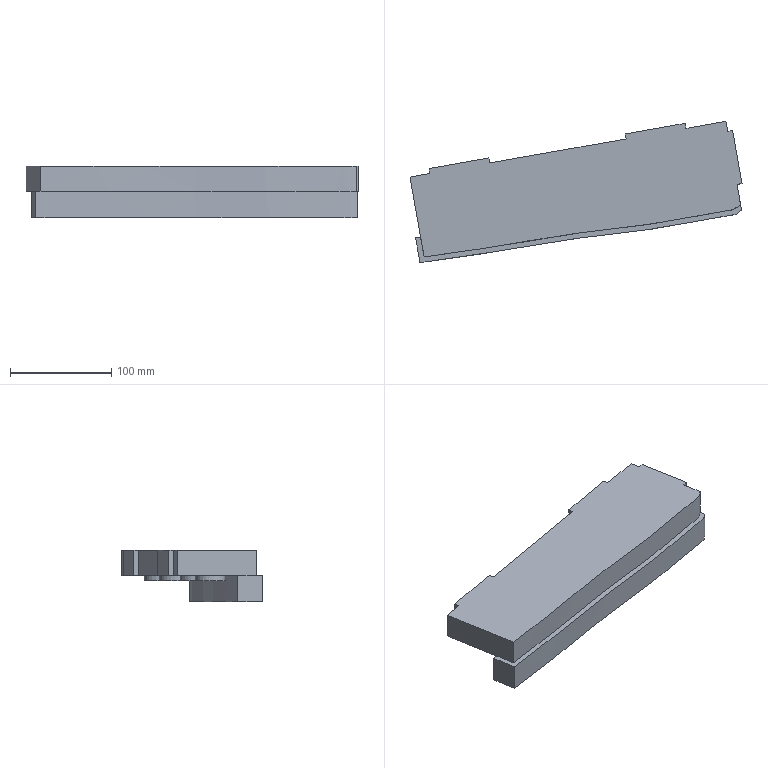Part | NX | features solid 2 | 1 solid | 33 faces | box 327.581 x 139.381 x 51 mm | volume 921541 mm3 | plane 25 | cylinder 5 | spline 3 | commonest cylinder face diameters 30 x5
STEP:
#1=CARTESIAN_POINT('',(309.963,629.515,45.));
#2=VERTEX_POINT('',#1);
#3=CARTESIAN_POINT('',(309.963,629.515,20.));
#4=VERTEX_POINT('',#3);
#5=CARTESIAN_POINT('',(309.963,629.515,51.));
#6=DIRECTION('',(0.,0.,-1.));
#7=VECTOR('',#6,1000.);
#8=LINE('',#5,#7);
#9=EDGE_CURVE('',#2,#4,#8,.T.);
#10=ORIENTED_EDGE('',*,*,#9,.F.);
#11=CARTESIAN_POINT('',(313.436,609.819,45.));
#12=VERTEX_POINT('',#11);
#13=CARTESIAN_POINT('',(310.85,624.485,45.));
#14=DIRECTION('',(-0.1736,0.9848,0.));
#15=VECTOR('',#14,1000.);
#16=LINE('',#13,#15);
#17=EDGE_CURVE('',#12,#2,#16,.T.);
#18=ORIENTED_EDGE('',*,*,#17,.F.);
#19=CARTESIAN_POINT('',(313.436,609.819,20.));
#20=VERTEX_POINT('',#19);
#21=CARTESIAN_POINT('',(313.436,609.819,32.5));
#22=DIRECTION('',(0.,0.,1.));
#23=VECTOR('',#22,1000.);
#24=LINE('',#21,#23);
#25=EDGE_CURVE('',#12,#20,#24,.F.);
#26=ORIENTED_EDGE('',*,*,#25,.T.);
#27=CARTESIAN_POINT('',(314.417,604.257,20.));
#28=VERTEX_POINT('',#27);
#29=CARTESIAN_POINT('',(314.417,604.257,20.));
#30=DIRECTION('',(0.1736,-0.9848,0.));
#31=VECTOR('',#30,1000.);
#32=LINE('',#29,#31);
#33=EDGE_CURVE('',#20,#28,#32,.T.);
#34=ORIENTED_EDGE('',*,*,#33,.T.);
#35=CARTESIAN_POINT('',(314.417,604.257,-6.));
#36=VERTEX_POINT('',#35);
#37=CARTESIAN_POINT('',(314.417,604.257,45.));
#38=DIRECTION('',(0.,0.,-1.));
#39=VECTOR('',#38,1000.);
#40=LINE('',#37,#39);
#41=EDGE_CURVE('',#28,#36,#40,.T.);
#42=ORIENTED_EDGE('',*,*,#41,.T.);
#43=CARTESIAN_POINT('',(310.85,624.485,-6.));
#44=VERTEX_POINT('',#43);
#45=CARTESIAN_POINT('',(314.417,604.257,-6.));
#46=DIRECTION('',(-0.1736,0.9848,0.));
#47=VECTOR('',#46,1000.);
#48=LINE('',#45,#47);
#49=EDGE_CURVE('',#36,#44,#48,.T.);
#50=ORIENTED_EDGE('',*,*,#49,.T.);
#51=CARTESIAN_POINT('',(310.85,624.485,20.));
#52=VERTEX_POINT('',#51);
#53=CARTESIAN_POINT('',(310.85,624.485,45.));
#54=DIRECTION('',(0.,0.,-1.));
#55=VECTOR('',#54,1000.);
#56=LINE('',#53,#55);
#57=EDGE_CURVE('',#52,#44,#56,.T.);
#58=ORIENTED_EDGE('',*,*,#57,.F.);
#59=CARTESIAN_POINT('',(310.85,624.485,20.));
#60=DIRECTION('',(-0.1736,0.9848,0.));
#61=VECTOR('',#60,1000.);
#62=LINE('',#59,#61);
#63=EDGE_CURVE('',#52,#4,#62,.T.);
#64=ORIENTED_EDGE('',*,*,#63,.T.);
#65=EDGE_LOOP('',(#10,#18,#26,#34,#42,#50,#58,#64));
#66=FACE_BOUND('',#65,.T.);
#67=CARTESIAN_POINT('',(310.85,624.485,51.));
#68=DIRECTION('',(-0.9848,-0.1736,0.));
#69=DIRECTION('',(0.1736,-0.9848,0.));
#70=AXIS2_PLACEMENT_3D('',#67,#68,#69);
#71=PLANE('',#70);
#72=ADVANCED_FACE('',(#66),#71,.F.);
#73=ORIENTED_EDGE('',*,*,#33,.F.);
#74=CARTESIAN_POINT('',(1.205,557.98,20.));
#75=VERTEX_POINT('',#74);
#76=CARTESIAN_POINT('',(1.205,557.98,20.));
#77=CARTESIAN_POINT('',(14.325,559.768,20.));
#78=CARTESIAN_POINT('',(40.557,563.408,20.));
#79=CARTESIAN_POINT('',(79.81,569.525,20.));
#80=CARTESIAN_POINT('',(118.938,576.402,20.));
#81=CARTESIAN_POINT('',(158.207,582.418,20.));
#82=CARTESIAN_POINT('',(191.141,586.056,20.));
#83=CARTESIAN_POINT('',(217.44,589.277,20.));
#84=CARTESIAN_POINT('',(237.09,592.203,20.));
#85=CARTESIAN_POINT('',(253.396,595.114,20.));
#86=CARTESIAN_POINT('',(266.419,597.584,20.));
#87=CARTESIAN_POINT('',(274.557,599.14,20.));
#88=CARTESIAN_POINT('',(281.071,600.358,20.));
#89=CARTESIAN_POINT('',(285.96,601.251,20.));
#90=CARTESIAN_POINT('',(290.854,602.116,20.));
#91=CARTESIAN_POINT('',(294.941,602.784,20.));
#92=CARTESIAN_POINT('',(298.218,603.269,20.));
#93=CARTESIAN_POINT('',(300.681,603.605,20.));
#94=CARTESIAN_POINT('',(302.738,603.855,20.));
#95=CARTESIAN_POINT('',(304.379,604.087,20.));
#96=CARTESIAN_POINT('',(305.604,604.285,20.));
#97=CARTESIAN_POINT('',(306.807,604.655,20.));
#98=CARTESIAN_POINT('',(307.753,605.393,20.));
#99=CARTESIAN_POINT('',(308.685,606.152,20.));
#100=CARTESIAN_POINT('',(310.582,607.623,20.));
#101=CARTESIAN_POINT('',(312.17,608.84,20.));
#102=CARTESIAN_POINT('',(313.436,609.819,20.));
#103=B_SPLINE_CURVE_WITH_KNOTS('',3,(#76,#77,#78,#79,#80,#81,#82,#83,#84,#85,#86,#87,#88,#89,#90,#91,#92,#93,#94,#95,#96,#97,#98,#99,#100,#101,#102),.UNSPECIFIED.,.F.,.F.,(4,1,1,1,1,1,1,1,1,1,1,1,1,1,1,1,1,1,1,1,1,1,1,1,4),(1.348,1.388,1.428,1.468,1.507,1.547,1.567,1.587,1.607,1.617,1.626,1.631,1.636,1.641,1.646,1.649,1.651,1.654,1.655,1.656,1.658,1.659,1.66,1.661,1.666),.UNSPECIFIED.);
#104=EDGE_CURVE('',#20,#75,#103,.F.);
#105=ORIENTED_EDGE('',*,*,#104,.T.);
#106=CARTESIAN_POINT('',(-2.273,577.703,20.));
#107=VERTEX_POINT('',#106);
#108=CARTESIAN_POINT('',(2.04,553.246,20.));
#109=DIRECTION('',(-0.1736,0.9848,0.));
#110=VECTOR('',#109,1000.);
#111=LINE('',#108,#110);
#112=EDGE_CURVE('',#75,#107,#111,.T.);
#113=ORIENTED_EDGE('',*,*,#112,.T.);
#114=CARTESIAN_POINT('',(-7.231,577.029,20.));
#115=VERTEX_POINT('',#114);
#116=CARTESIAN_POINT('',(-7.231,577.029,20.));
#117=CARTESIAN_POINT('',(-5.578,577.253,20.));
#118=CARTESIAN_POINT('',(-3.925,577.478,20.));
#119=CARTESIAN_POINT('',(-2.273,577.703,20.));
#120=B_SPLINE_CURVE_WITH_KNOTS('',3,(#116,#117,#118,#119),.UNSPECIFIED.,.F.,.F.,(4,4),(1.285,1.29),.UNSPECIFIED.);
#121=EDGE_CURVE('',#115,#107,#120,.T.);
#122=ORIENTED_EDGE('',*,*,#121,.F.);
#123=CARTESIAN_POINT('',(-2.884,552.378,20.));
#124=VERTEX_POINT('',#123);
#125=CARTESIAN_POINT('',(-2.884,552.378,20.));
#126=DIRECTION('',(0.1736,-0.9848,0.));
#127=VECTOR('',#126,1000.);
#128=LINE('',#125,#127);
#129=EDGE_CURVE('',#115,#124,#128,.T.);
#130=ORIENTED_EDGE('',*,*,#129,.T.);
#131=CARTESIAN_POINT('',(-2.884,552.378,20.));
#132=CARTESIAN_POINT('',(10.428,554.187,20.));
#133=CARTESIAN_POINT('',(37.046,557.843,20.));
#134=CARTESIAN_POINT('',(76.881,563.965,20.));
#135=CARTESIAN_POINT('',(116.588,570.919,20.));
#136=CARTESIAN_POINT('',(156.411,577.155,20.));
#137=CARTESIAN_POINT('',(189.82,580.881,20.));
#138=CARTESIAN_POINT('',(216.509,584.11,20.));
#139=CARTESIAN_POINT('',(236.457,587.028,20.));
#140=CARTESIAN_POINT('',(256.321,590.542,20.));
#141=CARTESIAN_POINT('',(272.836,593.737,20.));
#142=CARTESIAN_POINT('',(284.409,595.895,20.));
#143=CARTESIAN_POINT('',(291.032,597.073,20.));
#144=CARTESIAN_POINT('',(296.01,597.898,20.));
#145=CARTESIAN_POINT('',(300.172,598.501,20.));
#146=CARTESIAN_POINT('',(303.518,598.917,20.));
#147=CARTESIAN_POINT('',(306.008,599.248,20.));
#148=CARTESIAN_POINT('',(308.515,599.86,20.));
#149=CARTESIAN_POINT('',(310.577,601.196,20.));
#150=CARTESIAN_POINT('',(312.457,602.782,20.));
#151=CARTESIAN_POINT('',(313.77,603.756,20.));
#152=CARTESIAN_POINT('',(314.417,604.257,20.));
#153=B_SPLINE_CURVE_WITH_KNOTS('',3,(#131,#132,#133,#134,#135,#136,#137,#138,#139,#140,#141,#142,#143,#144,#145,#146,#147,#148,#149,#150,#151,#152),.UNSPECIFIED.,.F.,.F.,(4,1,1,1,1,1,1,1,1,1,1,1,1,1,1,1,1,1,1,4),(0.,0.0403,0.0806,0.1209,0.1612,0.2015,0.2217,0.2418,0.262,0.2821,0.2922,0.2972,0.3023,0.3073,0.3098,0.3123,0.3149,0.3174,0.3199,0.3224),.UNSPECIFIED.);
#154=EDGE_CURVE('',#124,#28,#153,.T.);
#155=ORIENTED_EDGE('',*,*,#154,.T.);
#156=EDGE_LOOP('',(#73,#105,#113,#122,#130,#155));
#157=FACE_BOUND('',#156,.T.);
#158=CARTESIAN_POINT('',(-48.851,534.884,20.));
#159=DIRECTION('',(0.,0.,1.));
#160=DIRECTION('',(1.,0.,0.));
#161=AXIS2_PLACEMENT_3D('',#158,#159,#160);
#162=PLANE('',#161);
#163=ADVANCED_FACE('',(#157),#162,.T.);
#164=CARTESIAN_POINT('',(-12.693,636.802,20.));
#165=VERTEX_POINT('',#164);
#166=CARTESIAN_POINT('',(2.04,553.246,20.));
#167=DIRECTION('',(-0.1736,0.9848,0.));
#168=VECTOR('',#167,1000.);
#169=LINE('',#166,#168);
#170=EDGE_CURVE('',#107,#165,#169,.T.);
#171=ORIENTED_EDGE('',*,*,#170,.T.);
#172=CARTESIAN_POINT('',(7.003,640.275,20.));
#173=VERTEX_POINT('',#172);
#174=CARTESIAN_POINT('',(-17.617,635.933,20.));
#175=DIRECTION('',(0.9848,0.1736,0.));
#176=VECTOR('',#175,1000.);
#177=LINE('',#174,#176);
#178=EDGE_CURVE('',#165,#173,#177,.T.);
#179=ORIENTED_EDGE('',*,*,#178,.T.);
#180=CARTESIAN_POINT('',(6.134,645.199,20.));
#181=VERTEX_POINT('',#180);
#182=CARTESIAN_POINT('',(6.134,645.199,20.));
#183=DIRECTION('',(0.1736,-0.9848,0.));
#184=VECTOR('',#183,1000.);
#185=LINE('',#182,#184);
#186=EDGE_CURVE('',#181,#173,#185,.T.);
#187=ORIENTED_EDGE('',*,*,#186,.F.);
#188=CARTESIAN_POINT('',(65.223,655.618,20.));
#189=VERTEX_POINT('',#188);
#190=CARTESIAN_POINT('',(-18.486,640.858,20.));
#191=DIRECTION('',(0.9848,0.1736,0.));
#192=VECTOR('',#191,1000.);
#193=LINE('',#190,#192);
#194=EDGE_CURVE('',#181,#189,#193,.T.);
#195=ORIENTED_EDGE('',*,*,#194,.T.);
#196=CARTESIAN_POINT('',(66.091,650.694,20.));
#197=VERTEX_POINT('',#196);
#198=CARTESIAN_POINT('',(65.223,655.618,20.));
#199=DIRECTION('',(0.1736,-0.9848,0.));
#200=VECTOR('',#199,1000.);
#201=LINE('',#198,#200);
#202=EDGE_CURVE('',#189,#197,#201,.T.);
#203=ORIENTED_EDGE('',*,*,#202,.T.);
#204=CARTESIAN_POINT('',(200.507,674.395,20.));
#205=VERTEX_POINT('',#204);
#206=CARTESIAN_POINT('',(-17.617,635.933,20.));
#207=DIRECTION('',(0.9848,0.1736,0.));
#208=VECTOR('',#207,1000.);
#209=LINE('',#206,#208);
#210=EDGE_CURVE('',#197,#205,#209,.T.);
#211=ORIENTED_EDGE('',*,*,#210,.T.);
#212=CARTESIAN_POINT('',(199.639,679.319,20.));
#213=VERTEX_POINT('',#212);
#214=CARTESIAN_POINT('',(211.511,611.988,20.));
#215=DIRECTION('',(0.1736,-0.9848,0.));
#216=VECTOR('',#215,1000.);
#217=LINE('',#214,#216);
#218=EDGE_CURVE('',#213,#205,#217,.T.);
#219=ORIENTED_EDGE('',*,*,#218,.F.);
#220=CARTESIAN_POINT('',(258.727,689.738,20.));
#221=VERTEX_POINT('',#220);
#222=CARTESIAN_POINT('',(214.411,681.923,20.));
#223=DIRECTION('',(0.9848,0.1736,0.));
#224=VECTOR('',#223,1000.);
#225=LINE('',#222,#224);
#226=EDGE_CURVE('',#213,#221,#225,.T.);
#227=ORIENTED_EDGE('',*,*,#226,.T.);
#228=CARTESIAN_POINT('',(259.595,684.814,20.));
#229=VERTEX_POINT('',#228);
#230=CARTESIAN_POINT('',(258.727,689.738,20.));
#231=DIRECTION('',(0.1736,-0.9848,0.));
#232=VECTOR('',#231,1000.);
#233=LINE('',#230,#232);
#234=EDGE_CURVE('',#221,#229,#233,.T.);
#235=ORIENTED_EDGE('',*,*,#234,.T.);
#236=CARTESIAN_POINT('',(298.988,691.76,20.));
#237=VERTEX_POINT('',#236);
#238=CARTESIAN_POINT('',(-17.617,635.933,20.));
#239=DIRECTION('',(0.9848,0.1736,0.));
#240=VECTOR('',#239,1000.);
#241=LINE('',#238,#240);
#242=EDGE_CURVE('',#229,#237,#241,.T.);
#243=ORIENTED_EDGE('',*,*,#242,.T.);
#244=CARTESIAN_POINT('',(300.724,681.911,20.));
#245=VERTEX_POINT('',#244);
#246=CARTESIAN_POINT('',(310.85,624.485,20.));
#247=DIRECTION('',(-0.1736,0.9848,0.));
#248=VECTOR('',#247,1000.);
#249=LINE('',#246,#248);
#250=EDGE_CURVE('',#245,#237,#249,.T.);
#251=ORIENTED_EDGE('',*,*,#250,.F.);
#252=CARTESIAN_POINT('',(305.648,682.78,20.));
#253=VERTEX_POINT('',#252);
#254=CARTESIAN_POINT('',(305.648,682.78,20.));
#255=DIRECTION('',(-0.9848,-0.1736,0.));
#256=VECTOR('',#255,1000.);
#257=LINE('',#254,#256);
#258=EDGE_CURVE('',#253,#245,#257,.T.);
#259=ORIENTED_EDGE('',*,*,#258,.F.);
#260=CARTESIAN_POINT('',(314.887,630.383,20.));
#261=VERTEX_POINT('',#260);
#262=CARTESIAN_POINT('',(315.774,625.353,20.));
#263=DIRECTION('',(-0.1736,0.9848,0.));
#264=VECTOR('',#263,1000.);
#265=LINE('',#262,#264);
#266=EDGE_CURVE('',#261,#253,#265,.T.);
#267=ORIENTED_EDGE('',*,*,#266,.F.);
#268=CARTESIAN_POINT('',(314.887,630.383,20.));
#269=DIRECTION('',(-0.9848,-0.1736,0.));
#270=VECTOR('',#269,1000.);
#271=LINE('',#268,#270);
#272=EDGE_CURVE('',#261,#4,#271,.T.);
#273=ORIENTED_EDGE('',*,*,#272,.T.);
#274=ORIENTED_EDGE('',*,*,#63,.F.);
#275=CARTESIAN_POINT('',(-2.273,577.703,20.));
#276=CARTESIAN_POINT('',(10.799,579.481,20.));
#277=CARTESIAN_POINT('',(36.932,583.099,20.));
#278=CARTESIAN_POINT('',(76.042,589.182,20.));
#279=CARTESIAN_POINT('',(115.028,596.001,20.));
#280=CARTESIAN_POINT('',(154.146,602.056,20.));
#281=CARTESIAN_POINT('',(186.932,605.717,20.));
#282=CARTESIAN_POINT('',(213.129,608.88,20.));
#283=CARTESIAN_POINT('',(232.711,611.745,20.));
#284=CARTESIAN_POINT('',(252.214,615.207,20.));
#285=CARTESIAN_POINT('',(271.682,618.983,20.));
#286=CARTESIAN_POINT('',(287.921,621.995,20.));
#287=CARTESIAN_POINT('',(300.971,623.881,20.));
#288=CARTESIAN_POINT('',(307.539,624.438,20.));
#289=CARTESIAN_POINT('',(310.85,624.485,20.));
#290=B_SPLINE_CURVE_WITH_KNOTS('',3,(#275,#276,#277,#278,#279,#280,#281,#282,#283,#284,#285,#286,#287,#288,#289),.UNSPECIFIED.,.F.,.F.,(4,1,1,1,1,1,1,1,1,1,1,1,4),(1.29,1.33,1.369,1.409,1.448,1.488,1.508,1.528,1.547,1.567,1.587,1.597,1.607),.UNSPECIFIED.);
#291=EDGE_CURVE('',#107,#52,#290,.T.);
#292=ORIENTED_EDGE('',*,*,#291,.F.);
#293=EDGE_LOOP('',(#171,#179,#187,#195,#203,#211,#219,#227,#235,#243,#251,#259,#267,#273,#274,#292));
#294=FACE_BOUND('',#293,.T.);
#295=CARTESIAN_POINT('',(70.617,619.28,20.));
#296=VERTEX_POINT('',#295);
#297=CARTESIAN_POINT('',(55.617,619.28,20.));
#298=DIRECTION('',(0.,0.,-1.));
#299=DIRECTION('',(1.,0.,0.));
#300=AXIS2_PLACEMENT_3D('',#297,#298,#299);
#301=CIRCLE('',#300,15.);
#302=EDGE_CURVE('',#296,#296,#301,.T.);
#303=ORIENTED_EDGE('',*,*,#302,.F.);
#304=EDGE_LOOP('',(#303));
#305=FACE_BOUND('',#304,.T.);
#306=CARTESIAN_POINT('',(35.617,604.28,20.));
#307=VERTEX_POINT('',#306);
#308=CARTESIAN_POINT('',(20.617,604.28,20.));
#309=DIRECTION('',(0.,0.,-1.));
#310=DIRECTION('',(1.,0.,0.));
#311=AXIS2_PLACEMENT_3D('',#308,#309,#310);
#312=CIRCLE('',#311,15.);
#313=EDGE_CURVE('',#307,#307,#312,.T.);
#314=ORIENTED_EDGE('',*,*,#313,.F.);
#315=EDGE_LOOP('',(#314));
#316=FACE_BOUND('',#315,.T.);
#317=CARTESIAN_POINT('',(155.617,639.28,20.));
#318=VERTEX_POINT('',#317);
#319=CARTESIAN_POINT('',(140.617,639.28,20.));
#320=DIRECTION('',(0.,0.,-1.));
#321=DIRECTION('',(1.,0.,0.));
#322=AXIS2_PLACEMENT_3D('',#319,#320,#321);
#323=CIRCLE('',#322,15.);
#324=EDGE_CURVE('',#318,#318,#323,.T.);
#325=ORIENTED_EDGE('',*,*,#324,.F.);
#326=EDGE_LOOP('',(#325));
#327=FACE_BOUND('',#326,.T.);
#328=CARTESIAN_POINT('',(285.617,644.28,20.));
#329=VERTEX_POINT('',#328);
#330=CARTESIAN_POINT('',(270.617,644.28,20.));
#331=DIRECTION('',(0.,0.,-1.));
#332=DIRECTION('',(1.,0.,0.));
#333=AXIS2_PLACEMENT_3D('',#330,#331,#332);
#334=CIRCLE('',#333,15.);
#335=EDGE_CURVE('',#329,#329,#334,.T.);
#336=ORIENTED_EDGE('',*,*,#335,.F.);
#337=EDGE_LOOP('',(#336));
#338=FACE_BOUND('',#337,.T.);
#339=CARTESIAN_POINT('',(250.617,654.28,20.));
#340=VERTEX_POINT('',#339);
#341=CARTESIAN_POINT('',(235.617,654.28,20.));
#342=DIRECTION('',(0.,0.,-1.));
#343=DIRECTION('',(1.,0.,0.));
#344=AXIS2_PLACEMENT_3D('',#341,#342,#343);
#345=CIRCLE('',#344,15.);
#346=EDGE_CURVE('',#340,#340,#345,.T.);
#347=ORIENTED_EDGE('',*,*,#346,.F.);
#348=EDGE_LOOP('',(#347));
#349=FACE_BOUND('',#348,.T.);
#350=CARTESIAN_POINT('',(-48.851,534.884,20.));
#351=DIRECTION('',(0.,0.,-1.));
#352=DIRECTION('',(-1.,0.,0.));
#353=AXIS2_PLACEMENT_3D('',#350,#351,#352);
#354=PLANE('',#353);
#355=ADVANCED_FACE('',(#294,#305,#316,#327,#338,#349),#354,.T.);
#356=CARTESIAN_POINT('',(199.639,679.319,45.));
#357=VERTEX_POINT('',#356);
#358=CARTESIAN_POINT('',(200.507,674.395,45.));
#359=VERTEX_POINT('',#358);
#360=CARTESIAN_POINT('',(211.511,611.988,45.));
#361=DIRECTION('',(0.1736,-0.9848,0.));
#362=VECTOR('',#361,1000.);
#363=LINE('',#360,#362);
#364=EDGE_CURVE('',#357,#359,#363,.T.);
#365=ORIENTED_EDGE('',*,*,#364,.T.);
#366=CARTESIAN_POINT('',(66.091,650.694,45.));
#367=VERTEX_POINT('',#366);
#368=CARTESIAN_POINT('',(-17.617,635.933,45.));
#369=DIRECTION('',(0.9848,0.1736,0.));
#370=VECTOR('',#369,1000.);
#371=LINE('',#368,#370);
#372=EDGE_CURVE('',#367,#359,#371,.T.);
#373=ORIENTED_EDGE('',*,*,#372,.F.);
#374=CARTESIAN_POINT('',(65.223,655.618,45.));
#375=VERTEX_POINT('',#374);
#376=CARTESIAN_POINT('',(65.223,655.618,45.));
#377=DIRECTION('',(0.1736,-0.9848,0.));
#378=VECTOR('',#377,1000.);
#379=LINE('',#376,#378);
#380=EDGE_CURVE('',#375,#367,#379,.T.);
#381=ORIENTED_EDGE('',*,*,#380,.F.);
#382=CARTESIAN_POINT('',(6.134,645.199,45.));
#383=VERTEX_POINT('',#382);
#384=CARTESIAN_POINT('',(-18.486,640.858,45.));
#385=DIRECTION('',(0.9848,0.1736,0.));
#386=VECTOR('',#385,1000.);
#387=LINE('',#384,#386);
#388=EDGE_CURVE('',#383,#375,#387,.T.);
#389=ORIENTED_EDGE('',*,*,#388,.F.);
#390=CARTESIAN_POINT('',(7.003,640.275,45.));
#391=VERTEX_POINT('',#390);
#392=CARTESIAN_POINT('',(6.134,645.199,45.));
#393=DIRECTION('',(0.1736,-0.9848,0.));
#394=VECTOR('',#393,1000.);
#395=LINE('',#392,#394);
#396=EDGE_CURVE('',#383,#391,#395,.T.);
#397=ORIENTED_EDGE('',*,*,#396,.T.);
#398=CARTESIAN_POINT('',(-12.693,636.802,45.));
#399=VERTEX_POINT('',#398);
#400=CARTESIAN_POINT('',(-17.617,635.933,45.));
#401=DIRECTION('',(0.9848,0.1736,0.));
#402=VECTOR('',#401,1000.);
#403=LINE('',#400,#402);
#404=EDGE_CURVE('',#399,#391,#403,.T.);
#405=ORIENTED_EDGE('',*,*,#404,.F.);
#406=CARTESIAN_POINT('',(1.205,557.98,45.));
#407=VERTEX_POINT('',#406);
#408=CARTESIAN_POINT('',(2.04,553.246,45.));
#409=DIRECTION('',(-0.1736,0.9848,0.));
#410=VECTOR('',#409,1000.);
#411=LINE('',#408,#410);
#412=EDGE_CURVE('',#407,#399,#411,.T.);
#413=ORIENTED_EDGE('',*,*,#412,.F.);
#414=CARTESIAN_POINT('',(313.436,609.819,45.));
#415=CARTESIAN_POINT('',(312.776,609.309,45.));
#416=CARTESIAN_POINT('',(311.443,608.269,45.));
#417=CARTESIAN_POINT('',(309.528,606.827,45.));
#418=CARTESIAN_POINT('',(307.273,604.992,45.));
#419=CARTESIAN_POINT('',(306.585,604.574,45.));
#420=CARTESIAN_POINT('',(305.305,604.21,45.));
#421=CARTESIAN_POINT('',(302.91,603.878,45.));
#422=CARTESIAN_POINT('',(300.438,603.574,45.));
#423=CARTESIAN_POINT('',(297.025,603.104,45.));
#424=CARTESIAN_POINT('',(292.837,602.451,45.));
#425=CARTESIAN_POINT('',(287.838,601.588,45.));
#426=CARTESIAN_POINT('',(282.889,600.693,45.));
#427=CARTESIAN_POINT('',(276.301,599.47,45.));
#428=CARTESIAN_POINT('',(268.097,597.906,45.));
#429=CARTESIAN_POINT('',(258.287,596.037,45.));
#430=CARTESIAN_POINT('',(248.489,594.24,45.));
#431=CARTESIAN_POINT('',(235.415,591.972,45.));
#432=CARTESIAN_POINT('',(219.064,589.495,45.));
#433=CARTESIAN_POINT('',(192.702,586.225,45.));
#434=CARTESIAN_POINT('',(159.458,582.584,45.));
#435=CARTESIAN_POINT('',(119.653,576.53,45.));
#436=CARTESIAN_POINT('',(80.253,569.598,45.));
#437=CARTESIAN_POINT('',(40.81,563.444,45.));
#438=CARTESIAN_POINT('',(14.419,559.781,45.));
#439=CARTESIAN_POINT('',(1.205,557.98,45.));
#440=B_SPLINE_CURVE_WITH_KNOTS('',3,(#414,#415,#416,#417,#418,#419,#420,#421,#422,#423,#424,#425,#426,#427,#428,#429,#430,#431,#432,#433,#434,#435,#436,#437,#438,#439),.UNSPECIFIED.,.F.,.F.,(4,1,1,1,1,1,1,1,1,1,1,1,1,1,1,1,1,1,1,1,1,1,1,4),(-0.00815,-0.0003902,0.007369,0.01513,0.02289,0.03065,0.03841,0.04617,0.05393,0.06945,0.08497,0.1005,0.116,0.147,0.1781,0.2091,0.2402,0.3022,0.3643,0.4885,0.6126,0.7368,0.8609,0.9851),.UNSPECIFIED.);
#441=EDGE_CURVE('',#12,#407,#440,.T.);
#442=ORIENTED_EDGE('',*,*,#441,.F.);
#443=ORIENTED_EDGE('',*,*,#17,.T.);
#444=CARTESIAN_POINT('',(314.887,630.383,45.));
#445=VERTEX_POINT('',#444);
#446=CARTESIAN_POINT('',(314.887,630.383,45.));
#447=DIRECTION('',(-0.9848,-0.1736,0.));
#448=VECTOR('',#447,1000.);
#449=LINE('',#446,#448);
#450=EDGE_CURVE('',#445,#2,#449,.T.);
#451=ORIENTED_EDGE('',*,*,#450,.F.);
#452=CARTESIAN_POINT('',(305.648,682.78,45.));
#453=VERTEX_POINT('',#452);
#454=CARTESIAN_POINT('',(315.774,625.353,45.));
#455=DIRECTION('',(-0.1736,0.9848,0.));
#456=VECTOR('',#455,1000.);
#457=LINE('',#454,#456);
#458=EDGE_CURVE('',#445,#453,#457,.T.);
#459=ORIENTED_EDGE('',*,*,#458,.T.);
#460=CARTESIAN_POINT('',(300.724,681.911,45.));
#461=VERTEX_POINT('',#460);
#462=CARTESIAN_POINT('',(305.648,682.78,45.));
#463=DIRECTION('',(-0.9848,-0.1736,0.));
#464=VECTOR('',#463,1000.);
#465=LINE('',#462,#464);
#466=EDGE_CURVE('',#453,#461,#465,.T.);
#467=ORIENTED_EDGE('',*,*,#466,.T.);
#468=CARTESIAN_POINT('',(298.988,691.76,45.));
#469=VERTEX_POINT('',#468);
#470=CARTESIAN_POINT('',(310.85,624.485,45.));
#471=DIRECTION('',(-0.1736,0.9848,0.));
#472=VECTOR('',#471,1000.);
#473=LINE('',#470,#472);
#474=EDGE_CURVE('',#461,#469,#473,.T.);
#475=ORIENTED_EDGE('',*,*,#474,.T.);
#476=CARTESIAN_POINT('',(259.595,684.814,45.));
#477=VERTEX_POINT('',#476);
#478=CARTESIAN_POINT('',(-17.617,635.933,45.));
#479=DIRECTION('',(0.9848,0.1736,0.));
#480=VECTOR('',#479,1000.);
#481=LINE('',#478,#480);
#482=EDGE_CURVE('',#477,#469,#481,.T.);
#483=ORIENTED_EDGE('',*,*,#482,.F.);
#484=CARTESIAN_POINT('',(258.727,689.738,45.));
#485=VERTEX_POINT('',#484);
#486=CARTESIAN_POINT('',(258.727,689.738,45.));
#487=DIRECTION('',(0.1736,-0.9848,0.));
#488=VECTOR('',#487,1000.);
#489=LINE('',#486,#488);
#490=EDGE_CURVE('',#485,#477,#489,.T.);
#491=ORIENTED_EDGE('',*,*,#490,.F.);
#492=CARTESIAN_POINT('',(214.411,681.923,45.));
#493=DIRECTION('',(0.9848,0.1736,0.));
#494=VECTOR('',#493,1000.);
#495=LINE('',#492,#494);
#496=EDGE_CURVE('',#357,#485,#495,.T.);
#497=ORIENTED_EDGE('',*,*,#496,.F.);
#498=EDGE_LOOP('',(#365,#373,#381,#389,#397,#405,#413,#442,#443,#451,#459,#467,#475,#483,#491,#497));
#499=FACE_BOUND('',#498,.T.);
#500=CARTESIAN_POINT('',(68.11,-778.743,45.));
#501=DIRECTION('',(0.,0.,1.));
#502=DIRECTION('',(1.,0.,0.));
#503=AXIS2_PLACEMENT_3D('',#500,#501,#502);
#504=PLANE('',#503);
#505=ADVANCED_FACE('',(#499),#504,.T.);
#506=CARTESIAN_POINT('',(-7.231,577.029,-6.));
#507=VERTEX_POINT('',#506);
#508=CARTESIAN_POINT('',(-7.231,577.029,-6.));
#509=CARTESIAN_POINT('',(3.216,578.448,-6.));
#510=CARTESIAN_POINT('',(32.842,582.473,-6.));
#511=CARTESIAN_POINT('',(80.9,589.874,-6.));
#512=CARTESIAN_POINT('',(129.178,598.51,-6.));
#513=CARTESIAN_POINT('',(168.762,603.734,-6.));
#514=CARTESIAN_POINT('',(197.885,606.967,-6.));
#515=CARTESIAN_POINT('',(225.861,610.552,-6.));
#516=CARTESIAN_POINT('',(253.734,615.432,-6.));
#517=CARTESIAN_POINT('',(281.075,620.874,-6.));
#518=CARTESIAN_POINT('',(302.687,624.369,-6.));
#519=CARTESIAN_POINT('',(310.85,624.485,-6.));
#520=B_SPLINE_CURVE_WITH_KNOTS('',3,(#508,#509,#510,#511,#512,#513,#514,#515,#516,#517,#518,#519),.UNSPECIFIED.,.F.,.F.,(4,1,1,1,1,1,1,1,1,4),(0.,0.09845,0.2798,0.4612,0.5518,0.6425,0.7332,0.8239,0.9146,1.),.UNSPECIFIED.);
#521=EDGE_CURVE('',#507,#44,#520,.T.);
#522=ORIENTED_EDGE('',*,*,#521,.T.);
#523=ORIENTED_EDGE('',*,*,#49,.F.);
#524=CARTESIAN_POINT('',(-2.884,552.378,-6.));
#525=VERTEX_POINT('',#524);
#526=CARTESIAN_POINT('',(314.417,604.257,-6.));
#527=CARTESIAN_POINT('',(313.456,603.513,-6.));
#528=CARTESIAN_POINT('',(311.997,602.42,-6.));
#529=CARTESIAN_POINT('',(310.125,600.866,-6.));
#530=CARTESIAN_POINT('',(308.006,599.638,-6.));
#531=CARTESIAN_POINT('',(304.985,599.087,-6.));
#532=CARTESIAN_POINT('',(297.755,598.23,-6.));
#533=CARTESIAN_POINT('',(282.167,595.571,-6.));
#534=CARTESIAN_POINT('',(258.333,590.865,-6.));
#535=CARTESIAN_POINT('',(229.601,585.825,-6.));
#536=CARTESIAN_POINT('',(200.669,582.121,-6.));
#537=CARTESIAN_POINT('',(171.683,578.904,-6.));
#538=CARTESIAN_POINT('',(142.767,575.084,-6.));
#539=CARTESIAN_POINT('',(113.981,570.414,-6.));
#540=CARTESIAN_POINT('',(85.244,565.431,-6.));
#541=CARTESIAN_POINT('',(56.452,560.795,-6.));
#542=CARTESIAN_POINT('',(27.599,556.541,-6.));
#543=CARTESIAN_POINT('',(7.807,553.831,-6.));
#544=CARTESIAN_POINT('',(-2.355,552.45,-6.));
#545=CARTESIAN_POINT('',(-2.884,552.378,-6.));
#546=B_SPLINE_CURVE_WITH_KNOTS('',3,(#526,#527,#528,#529,#530,#531,#532,#533,#534,#535,#536,#537,#538,#539,#540,#541,#542,#543,#544,#545),.UNSPECIFIED.,.F.,.F.,(4,1,1,1,1,1,1,1,1,1,1,1,1,1,1,1,1,4),(0.,0.01131,0.01696,0.02261,0.03392,0.04523,0.09046,0.1809,0.2714,0.3618,0.4523,0.5427,0.6332,0.7237,0.8141,0.9046,0.995,1.),.UNSPECIFIED.);
#547=EDGE_CURVE('',#36,#525,#546,.T.);
#548=ORIENTED_EDGE('',*,*,#547,.T.);
#549=CARTESIAN_POINT('',(-2.884,552.378,-6.));
#550=DIRECTION('',(-0.1736,0.9848,0.));
#551=VECTOR('',#550,1000.);
#552=LINE('',#549,#551);
#553=EDGE_CURVE('',#525,#507,#552,.T.);
#554=ORIENTED_EDGE('',*,*,#553,.T.);
#555=EDGE_LOOP('',(#522,#523,#548,#554));
#556=FACE_BOUND('',#555,.T.);
#557=CARTESIAN_POINT('',(68.11,-778.743,-6.));
#558=DIRECTION('',(0.,0.,1.));
#559=DIRECTION('',(1.,0.,0.));
#560=AXIS2_PLACEMENT_3D('',#557,#558,#559);
#561=PLANE('',#560);
#562=ADVANCED_FACE('',(#556),#561,.F.);
#563=CARTESIAN_POINT('',(125.617,639.28,15.));
#564=VERTEX_POINT('',#563);
#565=CARTESIAN_POINT('',(140.617,639.28,15.));
#566=DIRECTION('',(0.,0.,-1.));
#567=DIRECTION('',(-1.,0.,0.));
#568=AXIS2_PLACEMENT_3D('',#565,#566,#567);
#569=CIRCLE('',#568,15.);
#570=EDGE_CURVE('',#564,#564,#569,.T.);
#571=ORIENTED_EDGE('',*,*,#570,.T.);
#572=EDGE_LOOP('',(#571));
#573=FACE_BOUND('',#572,.T.);
#574=CARTESIAN_POINT('',(129.072,637.408,15.));
#575=DIRECTION('',(0.,0.,-1.));
#576=DIRECTION('',(-1.,0.,0.));
#577=AXIS2_PLACEMENT_3D('',#574,#575,#576);
#578=PLANE('',#577);
#579=ADVANCED_FACE('',(#573),#578,.T.);
#580=CARTESIAN_POINT('',(70.617,619.28,15.));
#581=VERTEX_POINT('',#580);
#582=CARTESIAN_POINT('',(55.617,619.28,15.));
#583=DIRECTION('',(0.,0.,-1.));
#584=DIRECTION('',(1.,0.,0.));
#585=AXIS2_PLACEMENT_3D('',#582,#583,#584);
#586=CIRCLE('',#585,15.);
#587=EDGE_CURVE('',#581,#581,#586,.T.);
#588=ORIENTED_EDGE('',*,*,#587,.T.);
#589=EDGE_LOOP('',(#588));
#590=FACE_BOUND('',#589,.T.);
#591=CARTESIAN_POINT('',(74.072,612.408,15.));
#592=DIRECTION('',(0.,0.,-1.));
#593=DIRECTION('',(-1.,0.,0.));
#594=AXIS2_PLACEMENT_3D('',#591,#592,#593);
#595=PLANE('',#594);
#596=ADVANCED_FACE('',(#590),#595,.T.);
#597=CARTESIAN_POINT('',(35.617,604.28,15.));
#598=VERTEX_POINT('',#597);
#599=CARTESIAN_POINT('',(20.617,604.28,15.));
#600=DIRECTION('',(0.,0.,-1.));
#601=DIRECTION('',(1.,0.,0.));
#602=AXIS2_PLACEMENT_3D('',#599,#600,#601);
#603=CIRCLE('',#602,15.);
#604=EDGE_CURVE('',#598,#598,#603,.T.);
#605=ORIENTED_EDGE('',*,*,#604,.T.);
#606=EDGE_LOOP('',(#605));
#607=FACE_BOUND('',#606,.T.);
#608=CARTESIAN_POINT('',(9.072,607.408,15.));
#609=DIRECTION('',(0.,0.,-1.));
#610=DIRECTION('',(-1.,0.,0.));
#611=AXIS2_PLACEMENT_3D('',#608,#609,#610);
#612=PLANE('',#611);
#613=ADVANCED_FACE('',(#607),#612,.T.);
#614=ORIENTED_EDGE('',*,*,#604,.F.);
#615=EDGE_LOOP('',(#614));
#616=FACE_BOUND('',#615,.T.);
#617=ORIENTED_EDGE('',*,*,#313,.T.);
#618=EDGE_LOOP('',(#617));
#619=FACE_BOUND('',#618,.T.);
#620=CARTESIAN_POINT('',(20.617,604.28,20.));
#621=DIRECTION('',(0.,0.,-1.));
#622=DIRECTION('',(-1.,0.,0.));
#623=AXIS2_PLACEMENT_3D('',#620,#621,#622);
#624=CYLINDRICAL_SURFACE('',#623,15.);
#625=ADVANCED_FACE('',(#616,#619),#624,.T.);
#626=ORIENTED_EDGE('',*,*,#587,.F.);
#627=EDGE_LOOP('',(#626));
#628=FACE_BOUND('',#627,.T.);
#629=ORIENTED_EDGE('',*,*,#302,.T.);
#630=EDGE_LOOP('',(#629));
#631=FACE_BOUND('',#630,.T.);
#632=CARTESIAN_POINT('',(55.617,619.28,20.));
#633=DIRECTION('',(0.,0.,-1.));
#634=DIRECTION('',(-1.,0.,0.));
#635=AXIS2_PLACEMENT_3D('',#632,#633,#634);
#636=CYLINDRICAL_SURFACE('',#635,15.);
#637=ADVANCED_FACE('',(#628,#631),#636,.T.);
#638=ORIENTED_EDGE('',*,*,#570,.F.);
#639=EDGE_LOOP('',(#638));
#640=FACE_BOUND('',#639,.T.);
#641=ORIENTED_EDGE('',*,*,#324,.T.);
#642=EDGE_LOOP('',(#641));
#643=FACE_BOUND('',#642,.T.);
#644=CARTESIAN_POINT('',(140.617,639.28,20.));
#645=DIRECTION('',(0.,0.,-1.));
#646=DIRECTION('',(-1.,0.,0.));
#647=AXIS2_PLACEMENT_3D('',#644,#645,#646);
#648=CYLINDRICAL_SURFACE('',#647,15.);
#649=ADVANCED_FACE('',(#640,#643),#648,.T.);
#650=ORIENTED_EDGE('',*,*,#412,.T.);
#651=CARTESIAN_POINT('',(-12.693,636.802,51.));
#652=DIRECTION('',(0.,0.,-1.));
#653=VECTOR('',#652,1000.);
#654=LINE('',#651,#653);
#655=EDGE_CURVE('',#399,#165,#654,.T.);
#656=ORIENTED_EDGE('',*,*,#655,.T.);
#657=ORIENTED_EDGE('',*,*,#170,.F.);
#658=ORIENTED_EDGE('',*,*,#112,.F.);
#659=CARTESIAN_POINT('',(1.205,557.98,32.5));
#660=DIRECTION('',(0.,0.,1.));
#661=VECTOR('',#660,1000.);
#662=LINE('',#659,#661);
#663=EDGE_CURVE('',#407,#75,#662,.F.);
#664=ORIENTED_EDGE('',*,*,#663,.F.);
#665=EDGE_LOOP('',(#650,#656,#657,#658,#664));
#666=FACE_BOUND('',#665,.T.);
#667=CARTESIAN_POINT('',(2.04,553.246,20.));
#668=DIRECTION('',(0.9848,0.1736,0.));
#669=DIRECTION('',(-0.1736,0.9848,0.));
#670=AXIS2_PLACEMENT_3D('',#667,#668,#669);
#671=PLANE('',#670);
#672=ADVANCED_FACE('',(#666),#671,.F.);
#673=ORIENTED_EDGE('',*,*,#129,.F.);
#674=CARTESIAN_POINT('',(-7.231,577.029,45.));
#675=DIRECTION('',(0.,0.,-1.));
#676=VECTOR('',#675,1000.);
#677=LINE('',#674,#676);
#678=EDGE_CURVE('',#115,#507,#677,.T.);
#679=ORIENTED_EDGE('',*,*,#678,.T.);
#680=ORIENTED_EDGE('',*,*,#553,.F.);
#681=CARTESIAN_POINT('',(-2.884,552.378,45.));
#682=DIRECTION('',(0.,0.,-1.));
#683=VECTOR('',#682,1000.);
#684=LINE('',#681,#683);
#685=EDGE_CURVE('',#124,#525,#684,.T.);
#686=ORIENTED_EDGE('',*,*,#685,.F.);
#687=EDGE_LOOP('',(#673,#679,#680,#686));
#688=FACE_BOUND('',#687,.T.);
#689=CARTESIAN_POINT('',(-7.231,577.029,51.));
#690=DIRECTION('',(-0.9848,-0.1736,0.));
#691=DIRECTION('',(0.1736,-0.9848,0.));
#692=AXIS2_PLACEMENT_3D('',#689,#690,#691);
#693=PLANE('',#692);
#694=ADVANCED_FACE('',(#688),#693,.T.);
#695=ORIENTED_EDGE('',*,*,#547,.F.);
#696=ORIENTED_EDGE('',*,*,#41,.F.);
#697=ORIENTED_EDGE('',*,*,#154,.F.);
#698=ORIENTED_EDGE('',*,*,#685,.T.);
#699=EDGE_LOOP('',(#695,#696,#697,#698));
#700=FACE_BOUND('',#699,.T.);
#701=CARTESIAN_POINT('',(314.417,604.257,20.));
#702=CARTESIAN_POINT('',(314.417,604.257,-6.));
#703=CARTESIAN_POINT('',(313.753,603.743,20.));
#704=CARTESIAN_POINT('',(313.753,603.743,-6.));
#705=CARTESIAN_POINT('',(312.402,602.744,20.));
#706=CARTESIAN_POINT('',(312.402,602.744,-6.));
#707=CARTESIAN_POINT('',(310.485,601.108,20.));
#708=CARTESIAN_POINT('',(310.485,601.108,-6.));
#709=CARTESIAN_POINT('',(308.318,599.78,20.));
#710=CARTESIAN_POINT('',(308.318,599.78,-6.));
#711=CARTESIAN_POINT('',(305.847,599.228,20.));
#712=CARTESIAN_POINT('',(305.847,599.228,-6.));
#713=CARTESIAN_POINT('',(303.339,598.893,20.));
#714=CARTESIAN_POINT('',(303.339,598.893,-6.));
#715=CARTESIAN_POINT('',(300.014,598.481,20.));
#716=CARTESIAN_POINT('',(300.014,598.481,-6.));
#717=CARTESIAN_POINT('',(295.861,597.874,20.));
#718=CARTESIAN_POINT('',(295.861,597.874,-6.));
#719=CARTESIAN_POINT('',(290.89,597.049,20.));
#720=CARTESIAN_POINT('',(290.89,597.049,-6.));
#721=CARTESIAN_POINT('',(284.273,595.869,20.));
#722=CARTESIAN_POINT('',(284.273,595.869,-6.));
#723=CARTESIAN_POINT('',(272.717,593.714,20.));
#724=CARTESIAN_POINT('',(272.717,593.714,-6.));
#725=CARTESIAN_POINT('',(256.235,590.526,20.));
#726=CARTESIAN_POINT('',(256.235,590.526,-6.));
#727=CARTESIAN_POINT('',(236.389,587.017,20.));
#728=CARTESIAN_POINT('',(236.389,587.017,-6.));
#729=CARTESIAN_POINT('',(216.451,584.102,20.));
#730=CARTESIAN_POINT('',(216.451,584.102,-6.));
#731=CARTESIAN_POINT('',(189.776,580.876,20.));
#732=CARTESIAN_POINT('',(189.776,580.876,-6.));
#733=CARTESIAN_POINT('',(156.395,577.152,20.));
#734=CARTESIAN_POINT('',(156.395,577.152,-6.));
#735=CARTESIAN_POINT('',(116.577,570.917,20.));
#736=CARTESIAN_POINT('',(116.577,570.917,-6.));
#737=CARTESIAN_POINT('',(76.878,563.964,20.));
#738=CARTESIAN_POINT('',(76.878,563.964,-6.));
#739=CARTESIAN_POINT('',(37.044,557.843,20.));
#740=CARTESIAN_POINT('',(37.044,557.843,-6.));
#741=CARTESIAN_POINT('',(10.427,554.187,20.));
#742=CARTESIAN_POINT('',(10.427,554.187,-6.));
#743=CARTESIAN_POINT('',(-2.884,552.378,20.));
#744=CARTESIAN_POINT('',(-2.884,552.378,-6.));
#745=B_SPLINE_SURFACE_WITH_KNOTS('',3,1,((#701,#702),(#703,#704),(#705,#706),(#707,#708),(#709,#710),(#711,#712),(#713,#714),(#715,#716),(#717,#718),(#719,#720),(#721,#722),(#723,#724),(#725,#726),(#727,#728),(#729,#730),(#731,#732),(#733,#734),(#735,#736),(#737,#738),(#739,#740),(#741,#742),(#743,#744)),.SURF_OF_LINEAR_EXTRUSION.,.F.,.F.,.F.,(4,1,1,1,1,1,1,1,1,1,1,1,1,1,1,1,1,1,1,4),(2,2),(0.,0.007812,0.01562,0.02344,0.03125,0.03906,0.04687,0.0625,0.07812,0.09375,0.125,0.1875,0.25,0.3125,0.375,0.5,0.625,0.75,0.875,1.),(0.,1.),.UNSPECIFIED.);
#746=ADVANCED_FACE('',(#700),#745,.T.);
#747=ORIENTED_EDGE('',*,*,#104,.F.);
#748=ORIENTED_EDGE('',*,*,#25,.F.);
#749=ORIENTED_EDGE('',*,*,#441,.T.);
#750=ORIENTED_EDGE('',*,*,#663,.T.);
#751=EDGE_LOOP('',(#747,#748,#749,#750));
#752=FACE_BOUND('',#751,.T.);
#753=CARTESIAN_POINT('',(313.436,609.819,20.));
#754=CARTESIAN_POINT('',(313.436,609.819,45.));
#755=CARTESIAN_POINT('',(312.776,609.309,20.));
#756=CARTESIAN_POINT('',(312.776,609.309,45.));
#757=CARTESIAN_POINT('',(311.443,608.269,20.));
#758=CARTESIAN_POINT('',(311.443,608.269,45.));
#759=CARTESIAN_POINT('',(309.528,606.827,20.));
#760=CARTESIAN_POINT('',(309.528,606.827,45.));
#761=CARTESIAN_POINT('',(307.273,604.992,20.));
#762=CARTESIAN_POINT('',(307.273,604.992,45.));
#763=CARTESIAN_POINT('',(306.585,604.574,20.));
#764=CARTESIAN_POINT('',(306.585,604.574,45.));
#765=CARTESIAN_POINT('',(305.305,604.21,20.));
#766=CARTESIAN_POINT('',(305.305,604.21,45.));
#767=CARTESIAN_POINT('',(302.91,603.878,20.));
#768=CARTESIAN_POINT('',(302.91,603.878,45.));
#769=CARTESIAN_POINT('',(300.438,603.574,20.));
#770=CARTESIAN_POINT('',(300.438,603.574,45.));
#771=CARTESIAN_POINT('',(297.025,603.104,20.));
#772=CARTESIAN_POINT('',(297.025,603.104,45.));
#773=CARTESIAN_POINT('',(292.837,602.451,20.));
#774=CARTESIAN_POINT('',(292.837,602.451,45.));
#775=CARTESIAN_POINT('',(287.838,601.588,20.));
#776=CARTESIAN_POINT('',(287.838,601.588,45.));
#777=CARTESIAN_POINT('',(282.889,600.693,20.));
#778=CARTESIAN_POINT('',(282.889,600.693,45.));
#779=CARTESIAN_POINT('',(276.301,599.47,20.));
#780=CARTESIAN_POINT('',(276.301,599.47,45.));
#781=CARTESIAN_POINT('',(268.097,597.906,20.));
#782=CARTESIAN_POINT('',(268.097,597.906,45.));
#783=CARTESIAN_POINT('',(258.287,596.037,20.));
#784=CARTESIAN_POINT('',(258.287,596.037,45.));
#785=CARTESIAN_POINT('',(248.489,594.24,20.));
#786=CARTESIAN_POINT('',(248.489,594.24,45.));
#787=CARTESIAN_POINT('',(235.415,591.972,20.));
#788=CARTESIAN_POINT('',(235.415,591.972,45.));
#789=CARTESIAN_POINT('',(219.064,589.495,20.));
#790=CARTESIAN_POINT('',(219.064,589.495,45.));
#791=CARTESIAN_POINT('',(192.702,586.225,20.));
#792=CARTESIAN_POINT('',(192.702,586.225,45.));
#793=CARTESIAN_POINT('',(159.458,582.584,20.));
#794=CARTESIAN_POINT('',(159.458,582.584,45.));
#795=CARTESIAN_POINT('',(119.653,576.53,20.));
#796=CARTESIAN_POINT('',(119.653,576.53,45.));
#797=CARTESIAN_POINT('',(80.253,569.598,20.));
#798=CARTESIAN_POINT('',(80.253,569.598,45.));
#799=CARTESIAN_POINT('',(40.81,563.444,20.));
#800=CARTESIAN_POINT('',(40.81,563.444,45.));
#801=CARTESIAN_POINT('',(14.419,559.781,20.));
#802=CARTESIAN_POINT('',(14.419,559.781,45.));
#803=CARTESIAN_POINT('',(1.205,557.98,20.));
#804=CARTESIAN_POINT('',(1.205,557.98,45.));
#805=B_SPLINE_SURFACE_WITH_KNOTS('',3,1,((#753,#754),(#755,#756),(#757,#758),(#759,#760),(#761,#762),(#763,#764),(#765,#766),(#767,#768),(#769,#770),(#771,#772),(#773,#774),(#775,#776),(#777,#778),(#779,#780),(#781,#782),(#783,#784),(#785,#786),(#787,#788),(#789,#790),(#791,#792),(#793,#794),(#795,#796),(#797,#798),(#799,#800),(#801,#802),(#803,#804)),.SURF_OF_LINEAR_EXTRUSION.,.F.,.F.,.F.,(4,1,1,1,1,1,1,1,1,1,1,1,1,1,1,1,1,1,1,1,1,1,1,4),(2,2),(-0.00815,-0.0003902,0.007369,0.01513,0.02289,0.03065,0.03841,0.04617,0.05393,0.06945,0.08497,0.1005,0.116,0.147,0.1781,0.2091,0.2402,0.3022,0.3643,0.4885,0.6126,0.7368,0.8609,0.9851),(0.,1.),.UNSPECIFIED.);
#806=ADVANCED_FACE('',(#752),#805,.F.);
#807=ORIENTED_EDGE('',*,*,#291,.T.);
#808=ORIENTED_EDGE('',*,*,#57,.T.);
#809=ORIENTED_EDGE('',*,*,#521,.F.);
#810=ORIENTED_EDGE('',*,*,#678,.F.);
#811=ORIENTED_EDGE('',*,*,#121,.T.);
#812=EDGE_LOOP('',(#807,#808,#809,#810,#811));
#813=FACE_BOUND('',#812,.T.);
#814=CARTESIAN_POINT('',(-7.231,577.029,20.));
#815=CARTESIAN_POINT('',(-7.231,577.029,-6.));
#816=CARTESIAN_POINT('',(6.034,578.831,20.));
#817=CARTESIAN_POINT('',(6.034,578.831,-6.));
#818=CARTESIAN_POINT('',(32.461,582.445,20.));
#819=CARTESIAN_POINT('',(32.461,582.445,-6.));
#820=CARTESIAN_POINT('',(71.624,588.456,20.));
#821=CARTESIAN_POINT('',(71.624,588.456,-6.));
#822=CARTESIAN_POINT('',(104.647,594.177,20.));
#823=CARTESIAN_POINT('',(104.647,594.177,-6.));
#824=CARTESIAN_POINT('',(131.444,598.575,20.));
#825=CARTESIAN_POINT('',(131.444,598.575,-6.));
#826=CARTESIAN_POINT('',(151.792,601.525,20.));
#827=CARTESIAN_POINT('',(151.792,601.525,-6.));
#828=CARTESIAN_POINT('',(172.171,604.083,20.));
#829=CARTESIAN_POINT('',(172.171,604.083,-6.));
#830=CARTESIAN_POINT('',(192.246,606.361,20.));
#831=CARTESIAN_POINT('',(192.246,606.361,-6.));
#832=CARTESIAN_POINT('',(211.788,608.71,20.));
#833=CARTESIAN_POINT('',(211.788,608.71,-6.));
#834=CARTESIAN_POINT('',(231.014,611.473,20.));
#835=CARTESIAN_POINT('',(231.014,611.473,-6.));
#836=CARTESIAN_POINT('',(247.043,614.277,20.));
#837=CARTESIAN_POINT('',(247.043,614.277,-6.));
#838=CARTESIAN_POINT('',(259.83,616.691,20.));
#839=CARTESIAN_POINT('',(259.83,616.691,-6.));
#840=CARTESIAN_POINT('',(269.56,618.563,20.));
#841=CARTESIAN_POINT('',(269.56,618.563,-6.));
#842=CARTESIAN_POINT('',(279.649,620.449,20.));
#843=CARTESIAN_POINT('',(279.649,620.449,-6.));
#844=CARTESIAN_POINT('',(290.439,622.36,20.));
#845=CARTESIAN_POINT('',(290.439,622.36,-6.));
#846=CARTESIAN_POINT('',(301.275,623.936,20.));
#847=CARTESIAN_POINT('',(301.275,623.936,-6.));
#848=CARTESIAN_POINT('',(307.865,624.442,20.));
#849=CARTESIAN_POINT('',(307.865,624.442,-6.));
#850=CARTESIAN_POINT('',(310.85,624.485,20.));
#851=CARTESIAN_POINT('',(310.85,624.485,-6.));
#852=B_SPLINE_SURFACE_WITH_KNOTS('',3,1,((#814,#815),(#816,#817),(#818,#819),(#820,#821),(#822,#823),(#824,#825),(#826,#827),(#828,#829),(#830,#831),(#832,#833),(#834,#835),(#836,#837),(#838,#839),(#840,#841),(#842,#843),(#844,#845),(#846,#847),(#848,#849),(#850,#851)),.SURF_OF_LINEAR_EXTRUSION.,.F.,.F.,.F.,(4,1,1,1,1,1,1,1,1,1,1,1,1,1,1,1,4),(2,2),(0.,0.125,0.25,0.375,0.4375,0.5,0.5625,0.625,0.6875,0.75,0.8125,0.8438,0.875,0.9062,0.9375,0.9688,1.),(0.,1.),.UNSPECIFIED.);
#853=ADVANCED_FACE('',(#813),#852,.T.);
#854=ORIENTED_EDGE('',*,*,#372,.T.);
#855=CARTESIAN_POINT('',(200.507,674.395,51.));
#856=DIRECTION('',(0.,0.,-1.));
#857=VECTOR('',#856,1000.);
#858=LINE('',#855,#857);
#859=EDGE_CURVE('',#359,#205,#858,.T.);
#860=ORIENTED_EDGE('',*,*,#859,.T.);
#861=ORIENTED_EDGE('',*,*,#210,.F.);
#862=CARTESIAN_POINT('',(66.091,650.694,51.));
#863=DIRECTION('',(0.,0.,-1.));
#864=VECTOR('',#863,1000.);
#865=LINE('',#862,#864);
#866=EDGE_CURVE('',#367,#197,#865,.T.);
#867=ORIENTED_EDGE('',*,*,#866,.F.);
#868=EDGE_LOOP('',(#854,#860,#861,#867));
#869=FACE_BOUND('',#868,.T.);
#870=CARTESIAN_POINT('',(-17.617,635.933,51.));
#871=DIRECTION('',(-0.1736,0.9848,0.));
#872=DIRECTION('',(-0.9848,-0.1736,0.));
#873=AXIS2_PLACEMENT_3D('',#870,#871,#872);
#874=PLANE('',#873);
#875=ADVANCED_FACE('',(#869),#874,.T.);
#876=CARTESIAN_POINT('',(199.639,679.319,51.));
#877=DIRECTION('',(0.,0.,-1.));
#878=VECTOR('',#877,1000.);
#879=LINE('',#876,#878);
#880=EDGE_CURVE('',#357,#213,#879,.T.);
#881=ORIENTED_EDGE('',*,*,#880,.F.);
#882=ORIENTED_EDGE('',*,*,#496,.T.);
#883=CARTESIAN_POINT('',(258.727,689.738,51.));
#884=DIRECTION('',(0.,0.,-1.));
#885=VECTOR('',#884,1000.);
#886=LINE('',#883,#885);
#887=EDGE_CURVE('',#485,#221,#886,.T.);
#888=ORIENTED_EDGE('',*,*,#887,.T.);
#889=ORIENTED_EDGE('',*,*,#226,.F.);
#890=EDGE_LOOP('',(#881,#882,#888,#889));
#891=FACE_BOUND('',#890,.T.);
#892=CARTESIAN_POINT('',(214.411,681.923,51.));
#893=DIRECTION('',(-0.1736,0.9848,0.));
#894=DIRECTION('',(-0.9848,-0.1736,0.));
#895=AXIS2_PLACEMENT_3D('',#892,#893,#894);
#896=PLANE('',#895);
#897=ADVANCED_FACE('',(#891),#896,.T.);
#898=CARTESIAN_POINT('',(259.595,684.814,51.));
#899=DIRECTION('',(0.,0.,-1.));
#900=VECTOR('',#899,1000.);
#901=LINE('',#898,#900);
#902=EDGE_CURVE('',#477,#229,#901,.T.);
#903=ORIENTED_EDGE('',*,*,#902,.T.);
#904=ORIENTED_EDGE('',*,*,#234,.F.);
#905=ORIENTED_EDGE('',*,*,#887,.F.);
#906=ORIENTED_EDGE('',*,*,#490,.T.);
#907=EDGE_LOOP('',(#903,#904,#905,#906));
#908=FACE_BOUND('',#907,.T.);
#909=CARTESIAN_POINT('',(258.727,689.738,51.));
#910=DIRECTION('',(-0.9848,-0.1736,0.));
#911=DIRECTION('',(0.1736,-0.9848,0.));
#912=AXIS2_PLACEMENT_3D('',#909,#910,#911);
#913=PLANE('',#912);
#914=ADVANCED_FACE('',(#908),#913,.F.);
#915=ORIENTED_EDGE('',*,*,#859,.F.);
#916=ORIENTED_EDGE('',*,*,#364,.F.);
#917=ORIENTED_EDGE('',*,*,#880,.T.);
#918=ORIENTED_EDGE('',*,*,#218,.T.);
#919=EDGE_LOOP('',(#915,#916,#917,#918));
#920=FACE_BOUND('',#919,.T.);
#921=CARTESIAN_POINT('',(199.639,679.319,51.));
#922=DIRECTION('',(-0.9848,-0.1736,0.));
#923=DIRECTION('',(0.1736,-0.9848,0.));
#924=AXIS2_PLACEMENT_3D('',#921,#922,#923);
#925=PLANE('',#924);
#926=ADVANCED_FACE('',(#920),#925,.T.);
#927=CARTESIAN_POINT('',(250.617,654.28,15.));
#928=VERTEX_POINT('',#927);
#929=CARTESIAN_POINT('',(235.617,654.28,15.));
#930=DIRECTION('',(0.,0.,-1.));
#931=DIRECTION('',(1.,0.,0.));
#932=AXIS2_PLACEMENT_3D('',#929,#930,#931);
#933=CIRCLE('',#932,15.);
#934=EDGE_CURVE('',#928,#928,#933,.T.);
#935=ORIENTED_EDGE('',*,*,#934,.T.);
#936=EDGE_LOOP('',(#935));
#937=FACE_BOUND('',#936,.T.);
#938=CARTESIAN_POINT('',(235.617,654.28,15.));
#939=DIRECTION('',(0.,0.,-1.));
#940=DIRECTION('',(-1.,0.,0.));
#941=AXIS2_PLACEMENT_3D('',#938,#939,#940);
#942=PLANE('',#941);
#943=ADVANCED_FACE('',(#937),#942,.T.);
#944=ORIENTED_EDGE('',*,*,#346,.T.);
#945=EDGE_LOOP('',(#944));
#946=FACE_BOUND('',#945,.T.);
#947=ORIENTED_EDGE('',*,*,#934,.F.);
#948=EDGE_LOOP('',(#947));
#949=FACE_BOUND('',#948,.T.);
#950=CARTESIAN_POINT('',(235.617,654.28,20.));
#951=DIRECTION('',(0.,0.,-1.));
#952=DIRECTION('',(-1.,0.,0.));
#953=AXIS2_PLACEMENT_3D('',#950,#951,#952);
#954=CYLINDRICAL_SURFACE('',#953,15.);
#955=ADVANCED_FACE('',(#946,#949),#954,.T.);
#956=CARTESIAN_POINT('',(285.617,644.28,15.));
#957=VERTEX_POINT('',#956);
#958=CARTESIAN_POINT('',(270.617,644.28,15.));
#959=DIRECTION('',(0.,0.,-1.));
#960=DIRECTION('',(1.,0.,0.));
#961=AXIS2_PLACEMENT_3D('',#958,#959,#960);
#962=CIRCLE('',#961,15.);
#963=EDGE_CURVE('',#957,#957,#962,.T.);
#964=ORIENTED_EDGE('',*,*,#963,.T.);
#965=EDGE_LOOP('',(#964));
#966=FACE_BOUND('',#965,.T.);
#967=CARTESIAN_POINT('',(270.617,644.28,15.));
#968=DIRECTION('',(0.,0.,-1.));
#969=DIRECTION('',(-1.,0.,0.));
#970=AXIS2_PLACEMENT_3D('',#967,#968,#969);
#971=PLANE('',#970);
#972=ADVANCED_FACE('',(#966),#971,.T.);
#973=ORIENTED_EDGE('',*,*,#335,.T.);
#974=EDGE_LOOP('',(#973));
#975=FACE_BOUND('',#974,.T.);
#976=ORIENTED_EDGE('',*,*,#963,.F.);
#977=EDGE_LOOP('',(#976));
#978=FACE_BOUND('',#977,.T.);
#979=CARTESIAN_POINT('',(270.617,644.28,20.));
#980=DIRECTION('',(0.,0.,-1.));
#981=DIRECTION('',(-1.,0.,0.));
#982=AXIS2_PLACEMENT_3D('',#979,#980,#981);
#983=CYLINDRICAL_SURFACE('',#982,15.);
#984=ADVANCED_FACE('',(#975,#978),#983,.T.);
#985=ORIENTED_EDGE('',*,*,#474,.F.);
#986=CARTESIAN_POINT('',(300.724,681.911,51.));
#987=DIRECTION('',(0.,0.,-1.));
#988=VECTOR('',#987,1000.);
#989=LINE('',#986,#988);
#990=EDGE_CURVE('',#461,#245,#989,.T.);
#991=ORIENTED_EDGE('',*,*,#990,.T.);
#992=ORIENTED_EDGE('',*,*,#250,.T.);
#993=CARTESIAN_POINT('',(298.988,691.76,51.));
#994=DIRECTION('',(0.,0.,-1.));
#995=VECTOR('',#994,1000.);
#996=LINE('',#993,#995);
#997=EDGE_CURVE('',#469,#237,#996,.T.);
#998=ORIENTED_EDGE('',*,*,#997,.F.);
#999=EDGE_LOOP('',(#985,#991,#992,#998));
#1000=FACE_BOUND('',#999,.T.);
#1001=CARTESIAN_POINT('',(310.85,624.485,51.));
#1002=DIRECTION('',(-0.9848,-0.1736,0.));
#1003=DIRECTION('',(0.1736,-0.9848,0.));
#1004=AXIS2_PLACEMENT_3D('',#1001,#1002,#1003);
#1005=PLANE('',#1004);
#1006=ADVANCED_FACE('',(#1000),#1005,.F.);
#1007=ORIENTED_EDGE('',*,*,#242,.F.);
#1008=ORIENTED_EDGE('',*,*,#902,.F.);
#1009=ORIENTED_EDGE('',*,*,#482,.T.);
#1010=ORIENTED_EDGE('',*,*,#997,.T.);
#1011=EDGE_LOOP('',(#1007,#1008,#1009,#1010));
#1012=FACE_BOUND('',#1011,.T.);
#1013=CARTESIAN_POINT('',(-17.617,635.933,51.));
#1014=DIRECTION('',(-0.1736,0.9848,0.));
#1015=DIRECTION('',(-0.9848,-0.1736,0.));
#1016=AXIS2_PLACEMENT_3D('',#1013,#1014,#1015);
#1017=PLANE('',#1016);
#1018=ADVANCED_FACE('',(#1012),#1017,.T.);
#1019=ORIENTED_EDGE('',*,*,#866,.T.);
#1020=ORIENTED_EDGE('',*,*,#202,.F.);
#1021=CARTESIAN_POINT('',(65.223,655.618,51.));
#1022=DIRECTION('',(0.,0.,-1.));
#1023=VECTOR('',#1022,1000.);
#1024=LINE('',#1021,#1023);
#1025=EDGE_CURVE('',#375,#189,#1024,.T.);
#1026=ORIENTED_EDGE('',*,*,#1025,.F.);
#1027=ORIENTED_EDGE('',*,*,#380,.T.);
#1028=EDGE_LOOP('',(#1019,#1020,#1026,#1027));
#1029=FACE_BOUND('',#1028,.T.);
#1030=CARTESIAN_POINT('',(65.223,655.618,51.));
#1031=DIRECTION('',(-0.9848,-0.1736,0.));
#1032=DIRECTION('',(0.1736,-0.9848,0.));
#1033=AXIS2_PLACEMENT_3D('',#1030,#1031,#1032);
#1034=PLANE('',#1033);
#1035=ADVANCED_FACE('',(#1029),#1034,.F.);
#1036=CARTESIAN_POINT('',(6.134,645.199,51.));
#1037=DIRECTION('',(0.,0.,-1.));
#1038=VECTOR('',#1037,1000.);
#1039=LINE('',#1036,#1038);
#1040=EDGE_CURVE('',#383,#181,#1039,.T.);
#1041=ORIENTED_EDGE('',*,*,#1040,.F.);
#1042=ORIENTED_EDGE('',*,*,#388,.T.);
#1043=ORIENTED_EDGE('',*,*,#1025,.T.);
#1044=ORIENTED_EDGE('',*,*,#194,.F.);
#1045=EDGE_LOOP('',(#1041,#1042,#1043,#1044));
#1046=FACE_BOUND('',#1045,.T.);
#1047=CARTESIAN_POINT('',(-18.486,640.858,51.));
#1048=DIRECTION('',(-0.1736,0.9848,0.));
#1049=DIRECTION('',(-0.9848,-0.1736,0.));
#1050=AXIS2_PLACEMENT_3D('',#1047,#1048,#1049);
#1051=PLANE('',#1050);
#1052=ADVANCED_FACE('',(#1046),#1051,.T.);
#1053=CARTESIAN_POINT('',(7.003,640.275,51.));
#1054=DIRECTION('',(0.,0.,-1.));
#1055=VECTOR('',#1054,1000.);
#1056=LINE('',#1053,#1055);
#1057=EDGE_CURVE('',#391,#173,#1056,.T.);
#1058=ORIENTED_EDGE('',*,*,#1057,.F.);
#1059=ORIENTED_EDGE('',*,*,#396,.F.);
#1060=ORIENTED_EDGE('',*,*,#1040,.T.);
#1061=ORIENTED_EDGE('',*,*,#186,.T.);
#1062=EDGE_LOOP('',(#1058,#1059,#1060,#1061));
#1063=FACE_BOUND('',#1062,.T.);
#1064=CARTESIAN_POINT('',(6.134,645.199,51.));
#1065=DIRECTION('',(-0.9848,-0.1736,0.));
#1066=DIRECTION('',(0.1736,-0.9848,0.));
#1067=AXIS2_PLACEMENT_3D('',#1064,#1065,#1066);
#1068=PLANE('',#1067);
#1069=ADVANCED_FACE('',(#1063),#1068,.T.);
#1070=ORIENTED_EDGE('',*,*,#1057,.T.);
#1071=ORIENTED_EDGE('',*,*,#178,.F.);
#1072=ORIENTED_EDGE('',*,*,#655,.F.);
#1073=ORIENTED_EDGE('',*,*,#404,.T.);
#1074=EDGE_LOOP('',(#1070,#1071,#1072,#1073));
#1075=FACE_BOUND('',#1074,.T.);
#1076=CARTESIAN_POINT('',(-17.617,635.933,51.));
#1077=DIRECTION('',(-0.1736,0.9848,0.));
#1078=DIRECTION('',(-0.9848,-0.1736,0.));
#1079=AXIS2_PLACEMENT_3D('',#1076,#1077,#1078);
#1080=PLANE('',#1079);
#1081=ADVANCED_FACE('',(#1075),#1080,.T.);
#1082=ORIENTED_EDGE('',*,*,#990,.F.);
#1083=ORIENTED_EDGE('',*,*,#466,.F.);
#1084=CARTESIAN_POINT('',(305.648,682.78,51.));
#1085=DIRECTION('',(0.,0.,-1.));
#1086=VECTOR('',#1085,1000.);
#1087=LINE('',#1084,#1086);
#1088=EDGE_CURVE('',#453,#253,#1087,.T.);
#1089=ORIENTED_EDGE('',*,*,#1088,.T.);
#1090=ORIENTED_EDGE('',*,*,#258,.T.);
#1091=EDGE_LOOP('',(#1082,#1083,#1089,#1090));
#1092=FACE_BOUND('',#1091,.T.);
#1093=CARTESIAN_POINT('',(305.648,682.78,51.));
#1094=DIRECTION('',(-0.1736,0.9848,0.));
#1095=DIRECTION('',(-0.9848,-0.1736,0.));
#1096=AXIS2_PLACEMENT_3D('',#1093,#1094,#1095);
#1097=PLANE('',#1096);
#1098=ADVANCED_FACE('',(#1092),#1097,.T.);
#1099=ORIENTED_EDGE('',*,*,#450,.T.);
#1100=ORIENTED_EDGE('',*,*,#9,.T.);
#1101=ORIENTED_EDGE('',*,*,#272,.F.);
#1102=CARTESIAN_POINT('',(314.887,630.383,51.));
#1103=DIRECTION('',(0.,0.,-1.));
#1104=VECTOR('',#1103,1000.);
#1105=LINE('',#1102,#1104);
#1106=EDGE_CURVE('',#445,#261,#1105,.T.);
#1107=ORIENTED_EDGE('',*,*,#1106,.F.);
#1108=EDGE_LOOP('',(#1099,#1100,#1101,#1107));
#1109=FACE_BOUND('',#1108,.T.);
#1110=CARTESIAN_POINT('',(314.887,630.383,32.5));
#1111=DIRECTION('',(-0.1736,0.9848,0.));
#1112=DIRECTION('',(-0.9848,-0.1736,0.));
#1113=AXIS2_PLACEMENT_3D('',#1110,#1111,#1112);
#1114=PLANE('',#1113);
#1115=ADVANCED_FACE('',(#1109),#1114,.F.);
#1116=ORIENTED_EDGE('',*,*,#266,.T.);
#1117=ORIENTED_EDGE('',*,*,#1088,.F.);
#1118=ORIENTED_EDGE('',*,*,#458,.F.);
#1119=ORIENTED_EDGE('',*,*,#1106,.T.);
#1120=EDGE_LOOP('',(#1116,#1117,#1118,#1119));
#1121=FACE_BOUND('',#1120,.T.);
#1122=CARTESIAN_POINT('',(315.774,625.353,51.));
#1123=DIRECTION('',(-0.9848,-0.1736,0.));
#1124=DIRECTION('',(0.1736,-0.9848,0.));
#1125=AXIS2_PLACEMENT_3D('',#1122,#1123,#1124);
#1126=PLANE('',#1125);
#1127=ADVANCED_FACE('',(#1121),#1126,.F.);
#1128=CLOSED_SHELL('',(#72,#163,#355,#505,#562,#579,#596,#613,#625,#637,#649,#672,#694,#746,#806,#853,#875,#897,#914,#926,#943,#955,#972,#984,#1006,#1018,#1035,#1052,#1069,#1081,#1098,#1115,#1127));
#1129=MANIFOLD_SOLID_BREP('',#1128);
#1130=(LENGTH_UNIT()NAMED_UNIT(*)SI_UNIT(.MILLI.,.METRE.));
#1131=UNCERTAINTY_MEASURE_WITH_UNIT(LENGTH_MEASURE(0.0508),#1130,'','');
#1132=(NAMED_UNIT(*)PLANE_ANGLE_UNIT()SI_UNIT($,.RADIAN.));
#1133=(NAMED_UNIT(*)SI_UNIT($,.STERADIAN.)SOLID_ANGLE_UNIT());
#1134=(GEOMETRIC_REPRESENTATION_CONTEXT(3)GLOBAL_UNCERTAINTY_ASSIGNED_CONTEXT((#1131))GLOBAL_UNIT_ASSIGNED_CONTEXT((#1130,#1132,#1133))REPRESENTATION_CONTEXT('',''));
#1135=ADVANCED_BREP_SHAPE_REPRESENTATION('',(#1129),#1134);